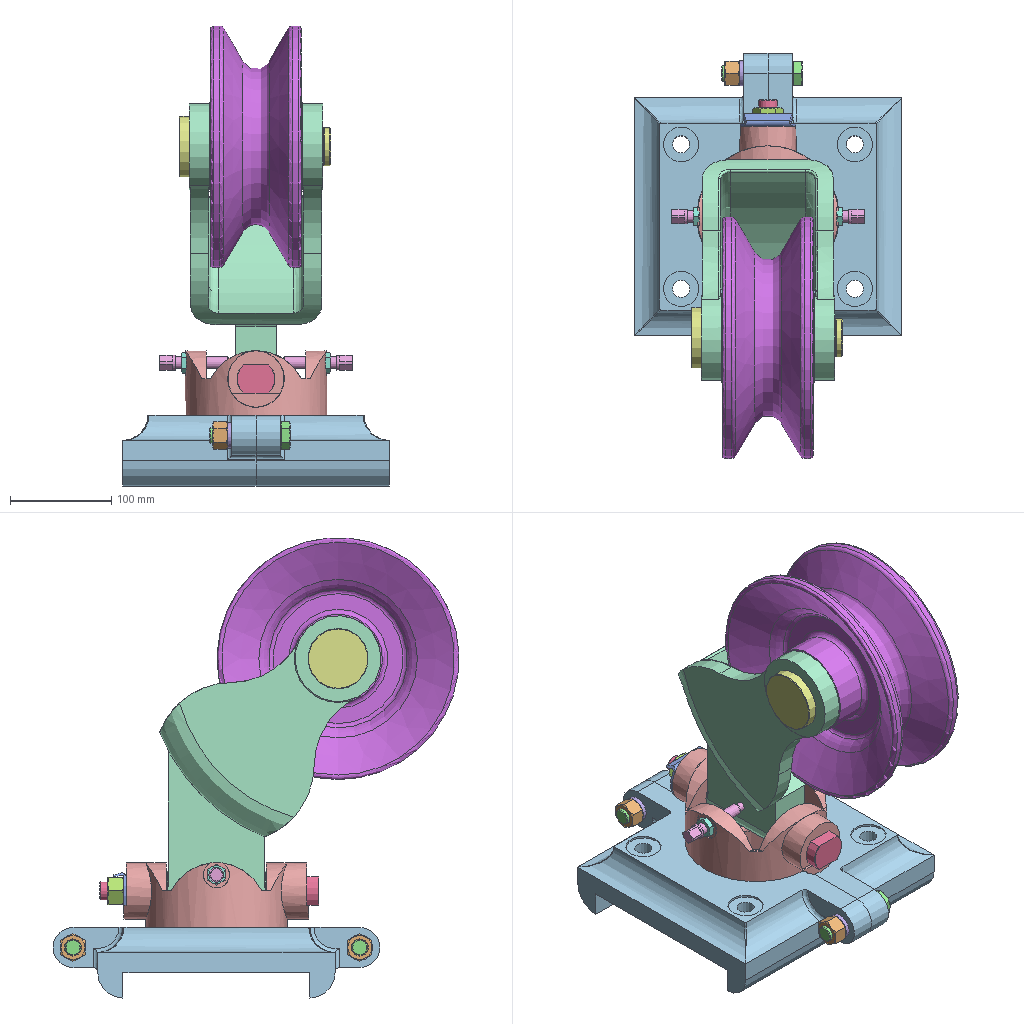Assembly | NX | 14 different items | 20 placed | box 264 x 402 x 455 mm
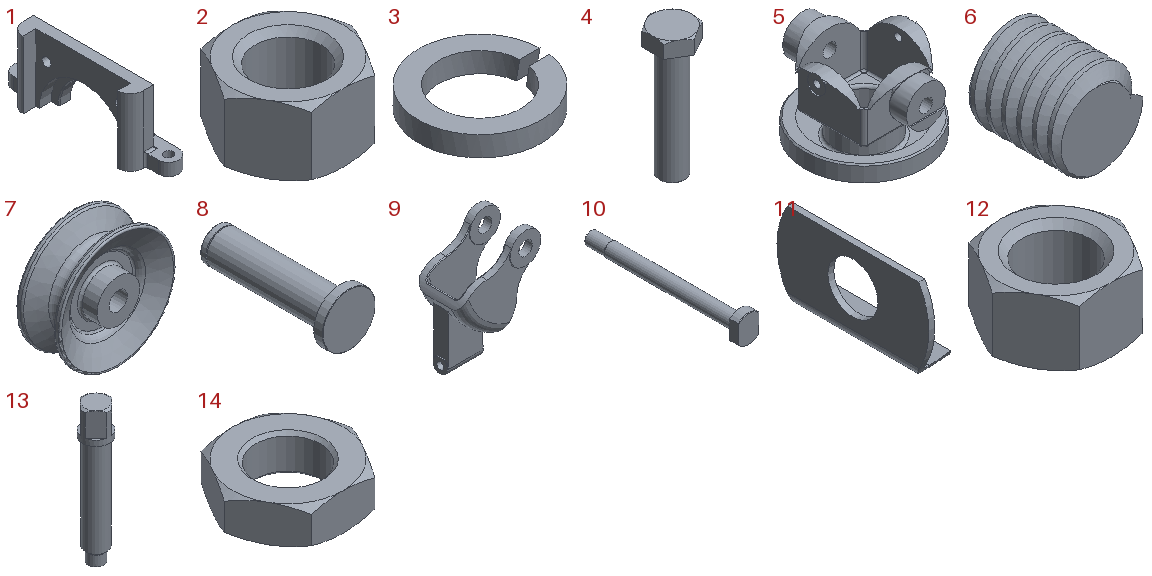Parts list (item | quantity | size | volume | features):
1 | x2 | 70 x 324 x 132 mm | 928360 mm3 | features DATUM_CSYS 8, SKETCH 7, EXTRUDE 5, BLEND 4, CBORE_HOLE 2, HOLE PACKAGE 2, SIMPLE HOLE 2, CHAMFER 1, SWP104 1
2 | x2 | 27.713 x 24 x 14.8 mm | 4858 mm3 | features META 3, SKETCH 3, DATUM_CSYS 2, EXTRUDE 2, SWP104 2, CHAMFER 1, LINE 1, SYMBOLIC_THREAD 1, THREADS 1
3 | x2 | 25.096 x 25.1 x 4.1 mm | 1074 mm3 | features DATUM_CSYS 2, SKETCH 2, EXTRUDE 1, LINE 1, META 1, SWP104 1
4 | x2 | 24 x 27.713 x 80 mm | 18388 mm3 | features SKETCH 4, EXTRUDE 3, META 3, DATUM_CSYS 2, BLEND 1, CHAMFER 1, LINE 1, SWP104 1, SYMBOLIC_THREAD 1, THREADS 1
5 | x1 | 172 x 182.995 x 109 mm | 961587 mm3 | features DATUM_CSYS 13, SKETCH 12, EXTRACT_DATUM_AXIS 10, EXTRUDE 9, EXTRACT_DATUM_PLANE 8, EXTRACT_FACE 6, HOLE PACKAGE 5, Instance Feature 5, EXTRACT_STRING 4, BLEND 3, SIMPLE HOLE 3, CBORE_HOLE 2, Intersection Curve 2, Mirror Feature 2, SYMBOLIC_THREAD 2, CHAMFER 1, DATUM_PLANE 1, Pattern Feature 1, SUBTRACT 1, SWP104 1
6 | x1 | 40 x 42 x 40 mm | 39845 mm3 | features DATUM_CSYS 2, CYLINDER 1, HELIX 1, SKETCH 1, SKIN 1, SUBTRACT 1
7 | x1 | 239.492 x 92 x 239.492 mm | 1529251 mm3 | features DATUM_CSYS 2, SKETCH 1, SWP104 1
8 | x1 | 60 x 150 x 60 mm | 186798 mm3 | features DATUM_CSYS 3, CHAMFER 2, SKETCH 2, SWP104 2, BLEND 1, Intersection Curve 1
9 | x1 | 219.007 x 132 x 292.5 mm | 1450063 mm3 | features DATUM_CSYS 8, BLEND 7, EXTRUDE 7, SKETCH 7, EXTRACT_FACE 4, CPROJ 2, EXTRACT_DATUM_AXIS 2, EXTRACT_DATUM_PLANE 2, HOLE PACKAGE 2, Instance Feature 2, Mirror Feature 2, SIMPLE HOLE 2, DATUM_PLANE 1
10 | x1 | 28 x 217 x 38 mm | 68775 mm3 | features DATUM_CSYS 3, CHAMFER 2, SKETCH 2, BLEND 1, EXTRUDE 1, SWP104 1, SYMBOLIC_THREAD 1
11 | x1 | 12.342 x 56 x 31.883 mm | 3985 mm3 | features DATUM_CSYS 3, EXTRUDE 2, SKETCH 2, HOLE PACKAGE 1, SIMPLE HOLE 1
12 | x1 | 31.177 x 27 x 15.8 mm | 6286 mm3 | features META 3, SKETCH 3, DATUM_CSYS 2, EXTRUDE 2, SWP104 2, CHAMFER 1, LINE 1, SYMBOLIC_THREAD 1, THREADS 1
13 | x2 | 14.7 x 14.7 x 76 mm | 8350 mm3 | features SKETCH 3, DATUM_CSYS 2, DATUM_PLANE 2, META 2, SWP104 2, EXTRUDE 1, LINE 1, SYMBOLIC_THREAD 1, THREADS 1
14 | x2 | 20.785 x 18 x 6 mm | 1134 mm3 | features META 3, SKETCH 3, DATUM_CSYS 2, EXTRUDE 2, SWP104 2, CHAMFER 1, LINE 1, SYMBOLIC_THREAD 1, THREADS 1
Mates (type | each side: item.copy, entity, surface, feature):
AlignLock | 7.1 face cylinder Revolve(1) | 9.1 face cylinder Ø38 Hole(9)
Center22 | 7.1 face plane Revolve(1) | 7.1 face plane Revolve(1) | 9.1 face plane Mirror Feature(8) | 9.1 face plane Extrude(7)
AlignLock | 8.1 edge | 9.1 edge
AlignLock | 1.1 face cylinder Revolve(5) | assembly axis
Touch | assembly plane | 1.1 face plane Extrude(6)
AlignLock | 1.1 edge | 1.1 edge
AlignLock | 1.1 edge | 4.1 edge
AlignLock | 3.1 edge | 1.1 edge | 2 times
AlignLock | 2.1 edge | 3.1 edge | 2 times
AlignLock | 4.1 edge | 1.1 edge
AlignLock | 13.1 face cylinder Revolve(6) | 14.1 face cylinder Extrude(8) | 2 times
Touch | 13.1 face sphere Revolve(6) | 9.1 face plane Mirror Feature(5)
Touch | 13.1 face sphere Revolve(6) | 9.1 face plane Extrude(4)
AlignLock | 10.1 face cylinder Revolve(1) | 12.1 face cylinder Extrude(6)
Touch | 11.1 face plane Extrude(1) | 12.1 face plane Extrude(5)